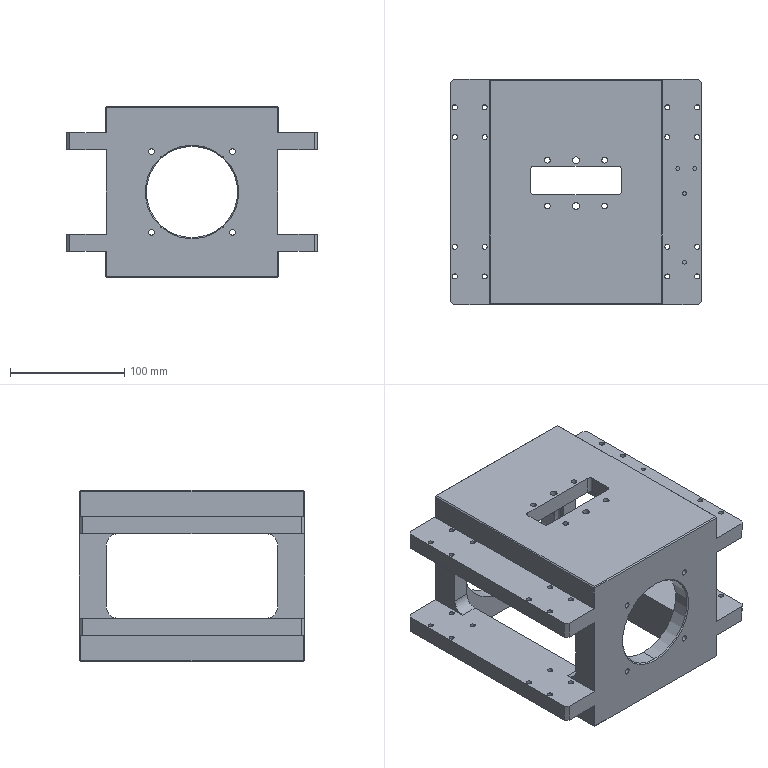Part | STEP file | 10-02 servo motor mounting seat | 1 solid | 216 faces | box 220 x 197 x 150 mm | volume 1555452 mm3 | cylinder 126 | plane 70 | cone 18 | spline 2 | commonest cylinder face diameters 4.5 x64 5 x28 3.3 x8 6 x8 20 x8 10 x6